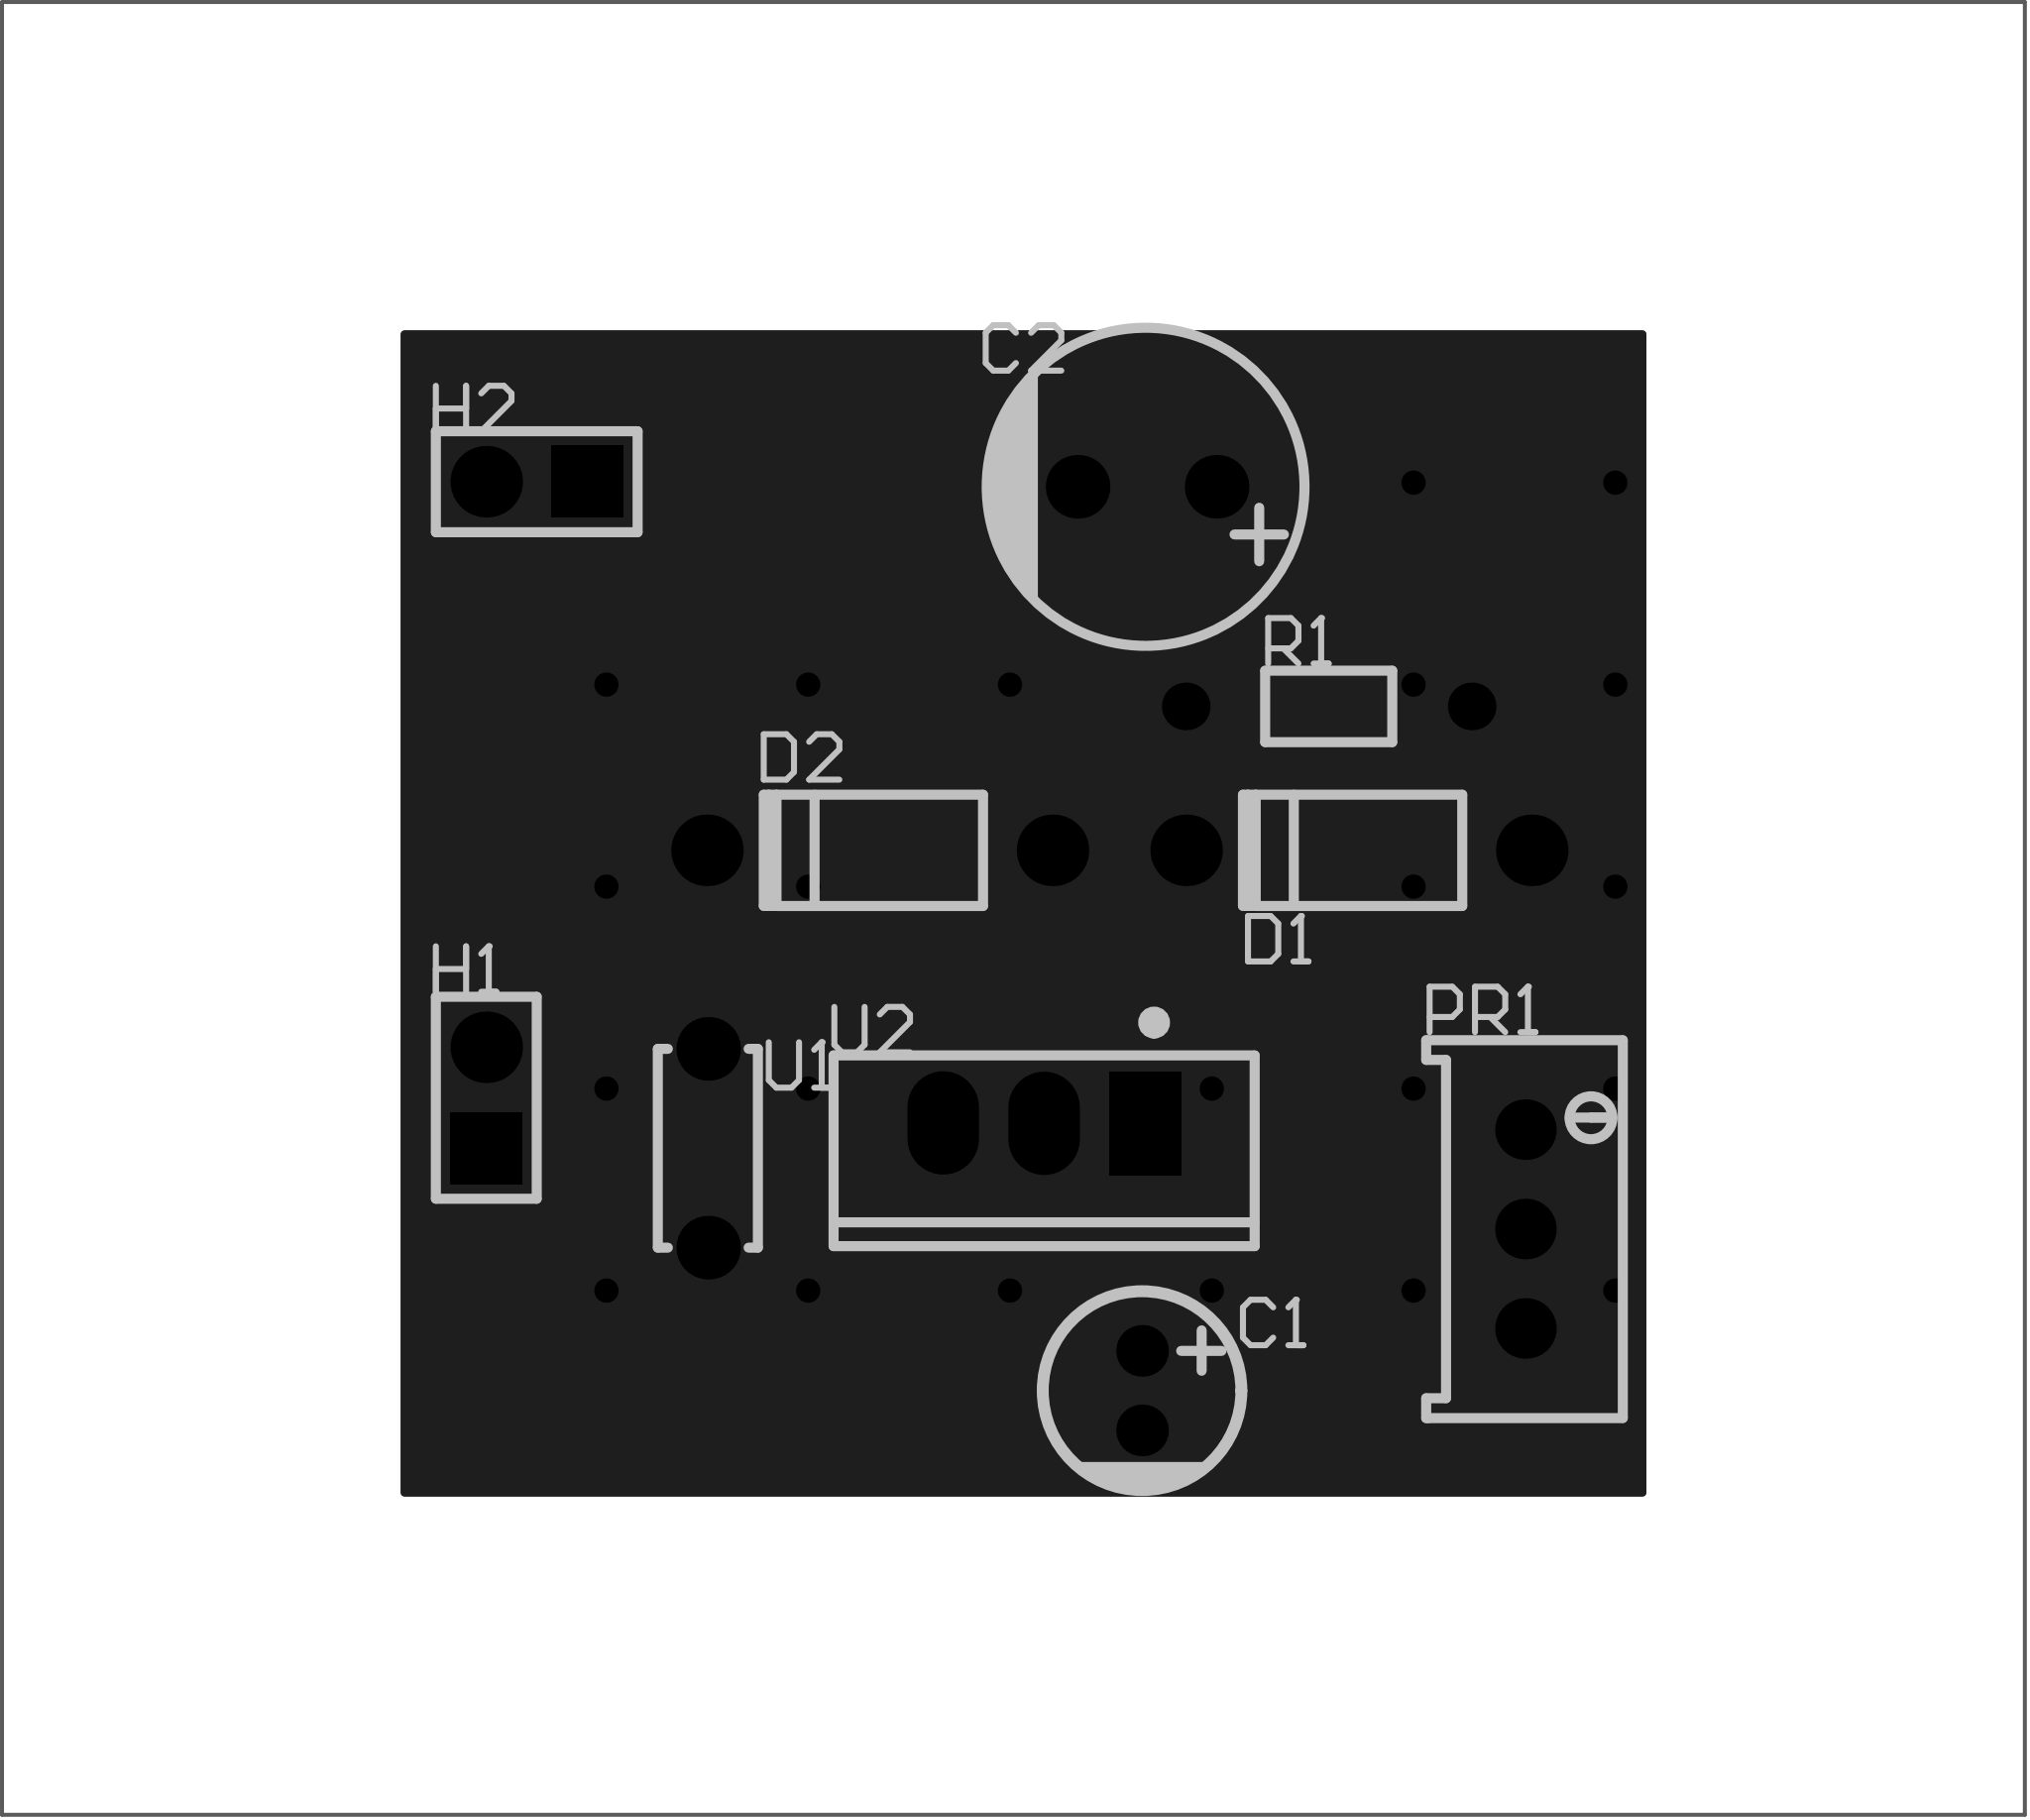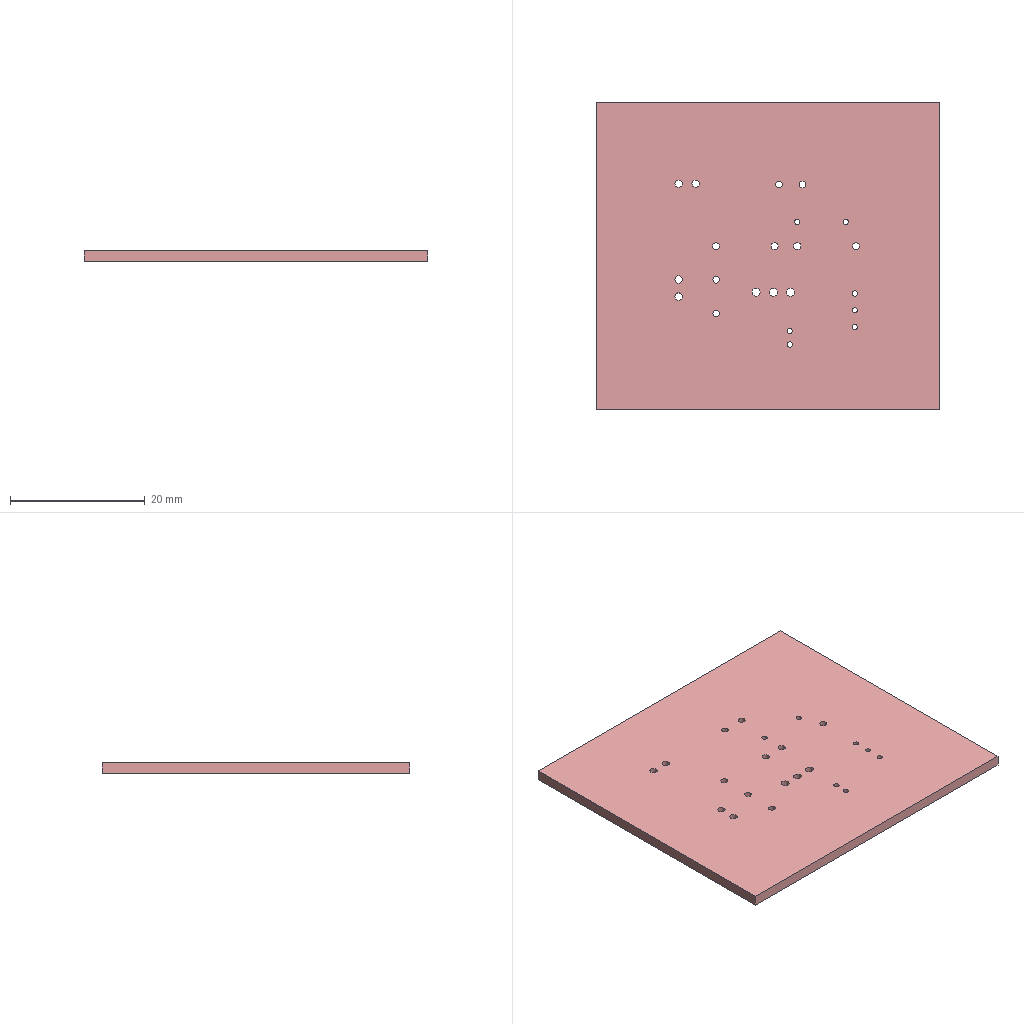Circuit board layout | Altium Designer | box 50.9 x 45.6 x 1.6 mm
Layer stack:
# Altium Designer layer stack of  (unit mm; dielectric type: 0 none, 1 core, 2 prepreg, 3 surface material)
index,name,kind,layer,copper_thickness_mm,dielectric_type,dielectric_thickness_mm,dielectric_material,dielectric_constant
0,Top Paste Mask Layer,other,,,,,,
1,Top Silkscreen Layer,other,,,,,,
2,Top Solder Mask Layer,dielectric,,,3,0.01,,3.3
3,Top Layer,copper,Top Layer,0.035,,,,
4,Dielectric1,dielectric,,,3,1.51,FR4,4.5
5,Bottom Layer,copper,Bottom Layer,0.035,,,,
6,Bottom Solder Mask Layer,dielectric,,,3,0.01,,3.3
7,Bottom Silkscreen Layer,other,,,,,,
8,Bottom Paste Mask Layer,other,,,,,,
# drill layer pairs: low layer,high layer
drill_pair,Top Layer,Bottom Layer
Part placement:
Designator,Comment,Layer,Footprint,Center-X(mm),Center-Y(mm),Rotation
C1,10uF,TopLayer,CAP-TH_BD5.0-P2.00-D0.8-FD-10UF50VC110GL,98.552,80.518,270
C2,100uF,TopLayer,CAP-TH_BD8.0-P3.50-D0.6-FD_1,98.679,103.251,180
D1,1N4001,TopLayer,DO-41_BD2.4-L4.7-P8.70-D0.8-RD,104.013,94.107,0
D2,1N4001,TopLayer,DO-41_BD2.4-L4.7-P8.70-D0.8-RD,91.948,94.107,0
H1,,TopLayer,HDR-TH_2P-P2.54-V-M-1,82.042,87.884,90
H2,,TopLayer,HDR-TH_2P-P2.54-V-M-1,83.312,103.378,180
PR1,10kΩ,TopLayer,R_3296,108.204,84.582,270
R1,200Ω,TopLayer,Res_1/8W,103.251,97.727,180
U1,2.2nF,TopLayer,CAP-TH_L5.0-W2.5-P5.00-D1.0,87.63,86.614,270
U2,LM317AHVT,TopLayer,TO-220-3_L10.0-W4.5-P2.54-L,96.086,87.246,180
Pad and via stacks:
# Altium Designer via and pad stacks of  (unit mm). Each distinct definition once, with the count of objects using it.
# via: kind,start_layer,end_layer,hole_mm,diameter_mm,mode(0 simple;1 top-mid-bottom;2 full stack),diameter_per_layer,count,example_net
# pad: kind,layer,hole_mm,hole_type(0 round;1 square;2 slot),plating,top_size,top_shape(1 round;2 rect;3 octagon;9 rounded rect),mid_size,bottom_size,mode,footprint,size_per_layer,count,example
pad,Multi-Layer,0.8,0,plated,1.3x1.3,1,1.3x1.3,1.3x1.3,0,CAP-TH_BD5.0-P2.00-D0.8-FD-10UF50VC110GL,,2,C1.2
pad,Multi-Layer,1,0,plated,1.6x1.6,1,1.6x1.6,1.6x1.6,0,CAP-TH_BD8.0-P3.50-D0.6-FD_1,,2,C2.2
pad,Multi-Layer,1.05,0,plated,1.8x1.8,1,1.8x1.8,1.8x1.8,0,DO-41_BD2.4-L4.7-P8.70-D0.8-RD,,4,D1.2
pad,Multi-Layer,1.1,0,plated,1.8x1.8,1,1.8x1.8,1.8x1.8,0,HDR-TH_2P-P2.54-V-M-1,,2,H1.2
pad,Multi-Layer,1.1,0,plated,1.8x1.8,2,1.8x1.8,1.8x1.8,0,HDR-TH_2P-P2.54-V-M-1,,2,H1.1
pad,Multi-Layer,0.762,0,plated,1.524x1.524,1,1.524x1.524,1.524x1.524,0,R_3296,,3,PR1.2
pad,Multi-Layer,0.8001,0,plated,1.199x1.199,1,1.199x1.199,1.199x1.199,0,Res_1/8W,,2,R1.1
pad,Multi-Layer,1,0,plated,1.6x1.6,1,1.6x1.6,1.6x1.6,0,CAP-TH_L5.0-W2.5-P5.00-D1.0,,2,U1.1
pad,Multi-Layer,1.2,0,plated,1.8x2.6,1,1.8x2.6,1.8x2.6,0,TO-220-3_L10.0-W4.5-P2.54-L,,2,U2.2
pad,Multi-Layer,1.2,0,plated,1.8x2.6,2,1.8x2.6,1.8x2.6,0,TO-220-3_L10.0-W4.5-P2.54-L,,1,U2.1
via,Top Layer,Bottom Layer,0.3048,0.61,0,,23,GND
Copper pours:
name,layer,net,type(0 solid;1 hatched;2 none)
Top Layer-GND,Top Layer,GND,0
Bottom Layer-GND,Bottom Layer,GND,0